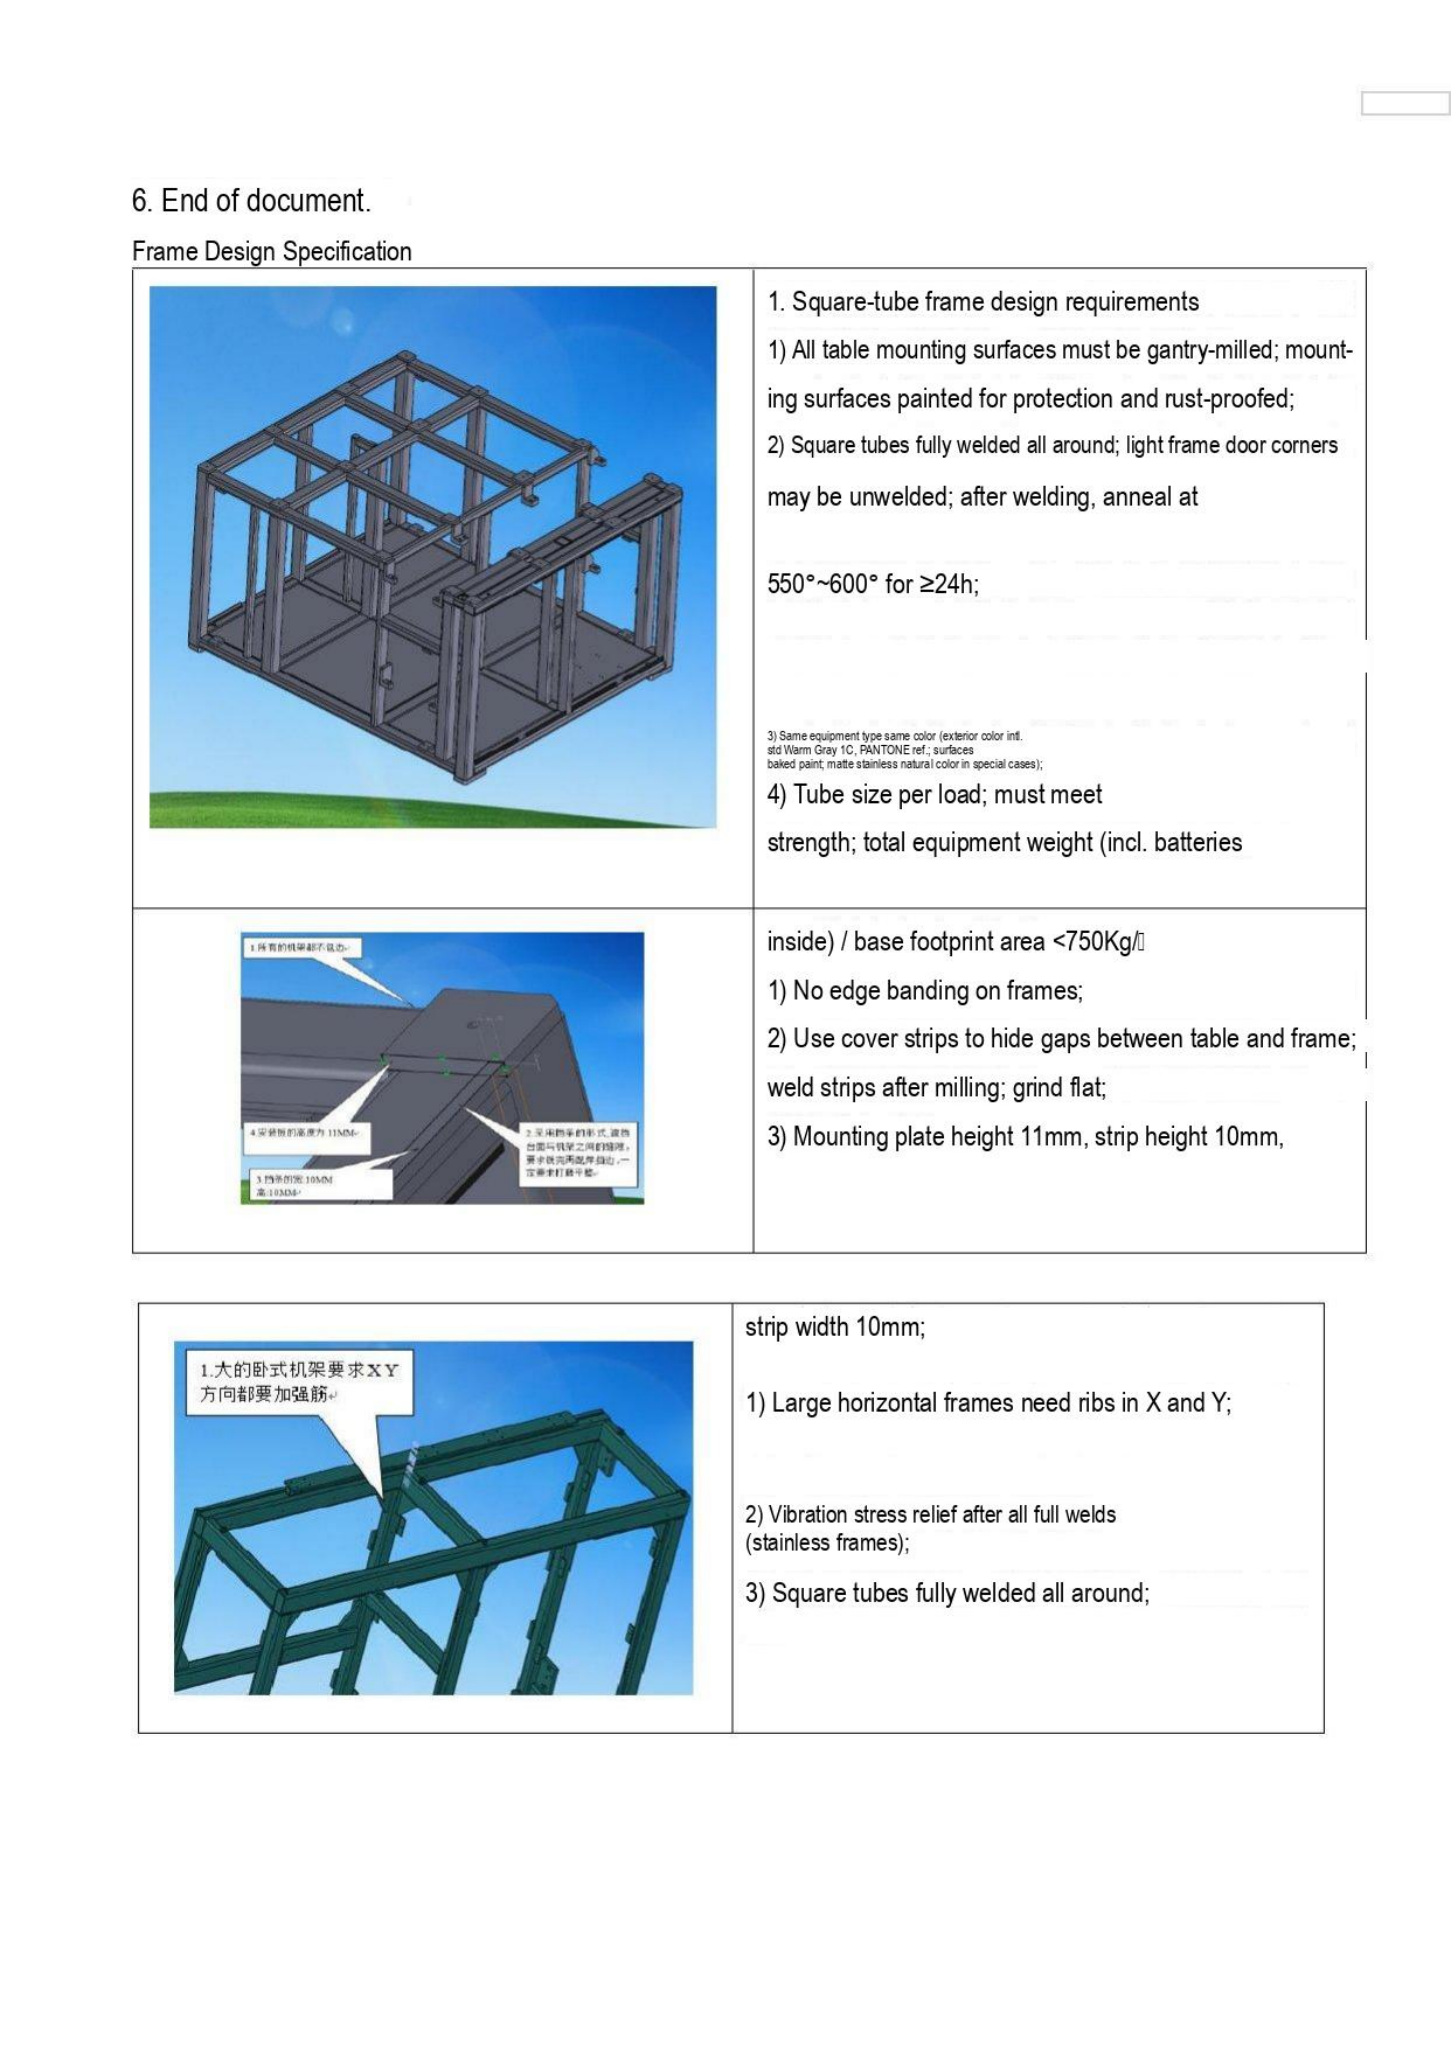6. End of document.

Frame Design Specification

| | |
|---|---|
| | 1. Square-tube frame design requirements<br>1) All table mounting surfaces must be gantry-milled; mounting surfaces painted for protection and rust-proofed;<br>2) Square tubes fully welded all around; light frame door corners may be unwelded; after welding, anneal at 550°~600° for ≥24h;<br>3) Same equipment type same color (exterior color inf. std Warm Gray 1C, PANTONE ref.; surfaces baked paint; matte stainless natural color in special cases);<br>4) Tube size per load; must meet strength; total equipment weight (incl. batteries |
| 1.所有的机架都不包边<br>4.安装板的高度为11MM<br>3.挡条的宽10MM 高10MM<br>2.采用挡条的形式,遮挡台面与机架之间的缝隙,要求铣完再焊挡条,一定要求打磨平整 | inside) / base footprint area <750Kg/<br>1) No edge banding on frames;<br>2) Use cover strips to hide gaps between table and frame; weld strips after milling; grind flat;<br>3) Mounting plate height 11mm, strip height 10mm, |

| | |
|---|---|
| 1.大的卧式机架要求XY方向都要加强筋 | strip width 10mm;<br>1) Large horizontal frames need ribs in X and Y;<br>2) Vibration stress relief after all full welds (stainless frames);<br>3) Square tubes fully welded all around; |
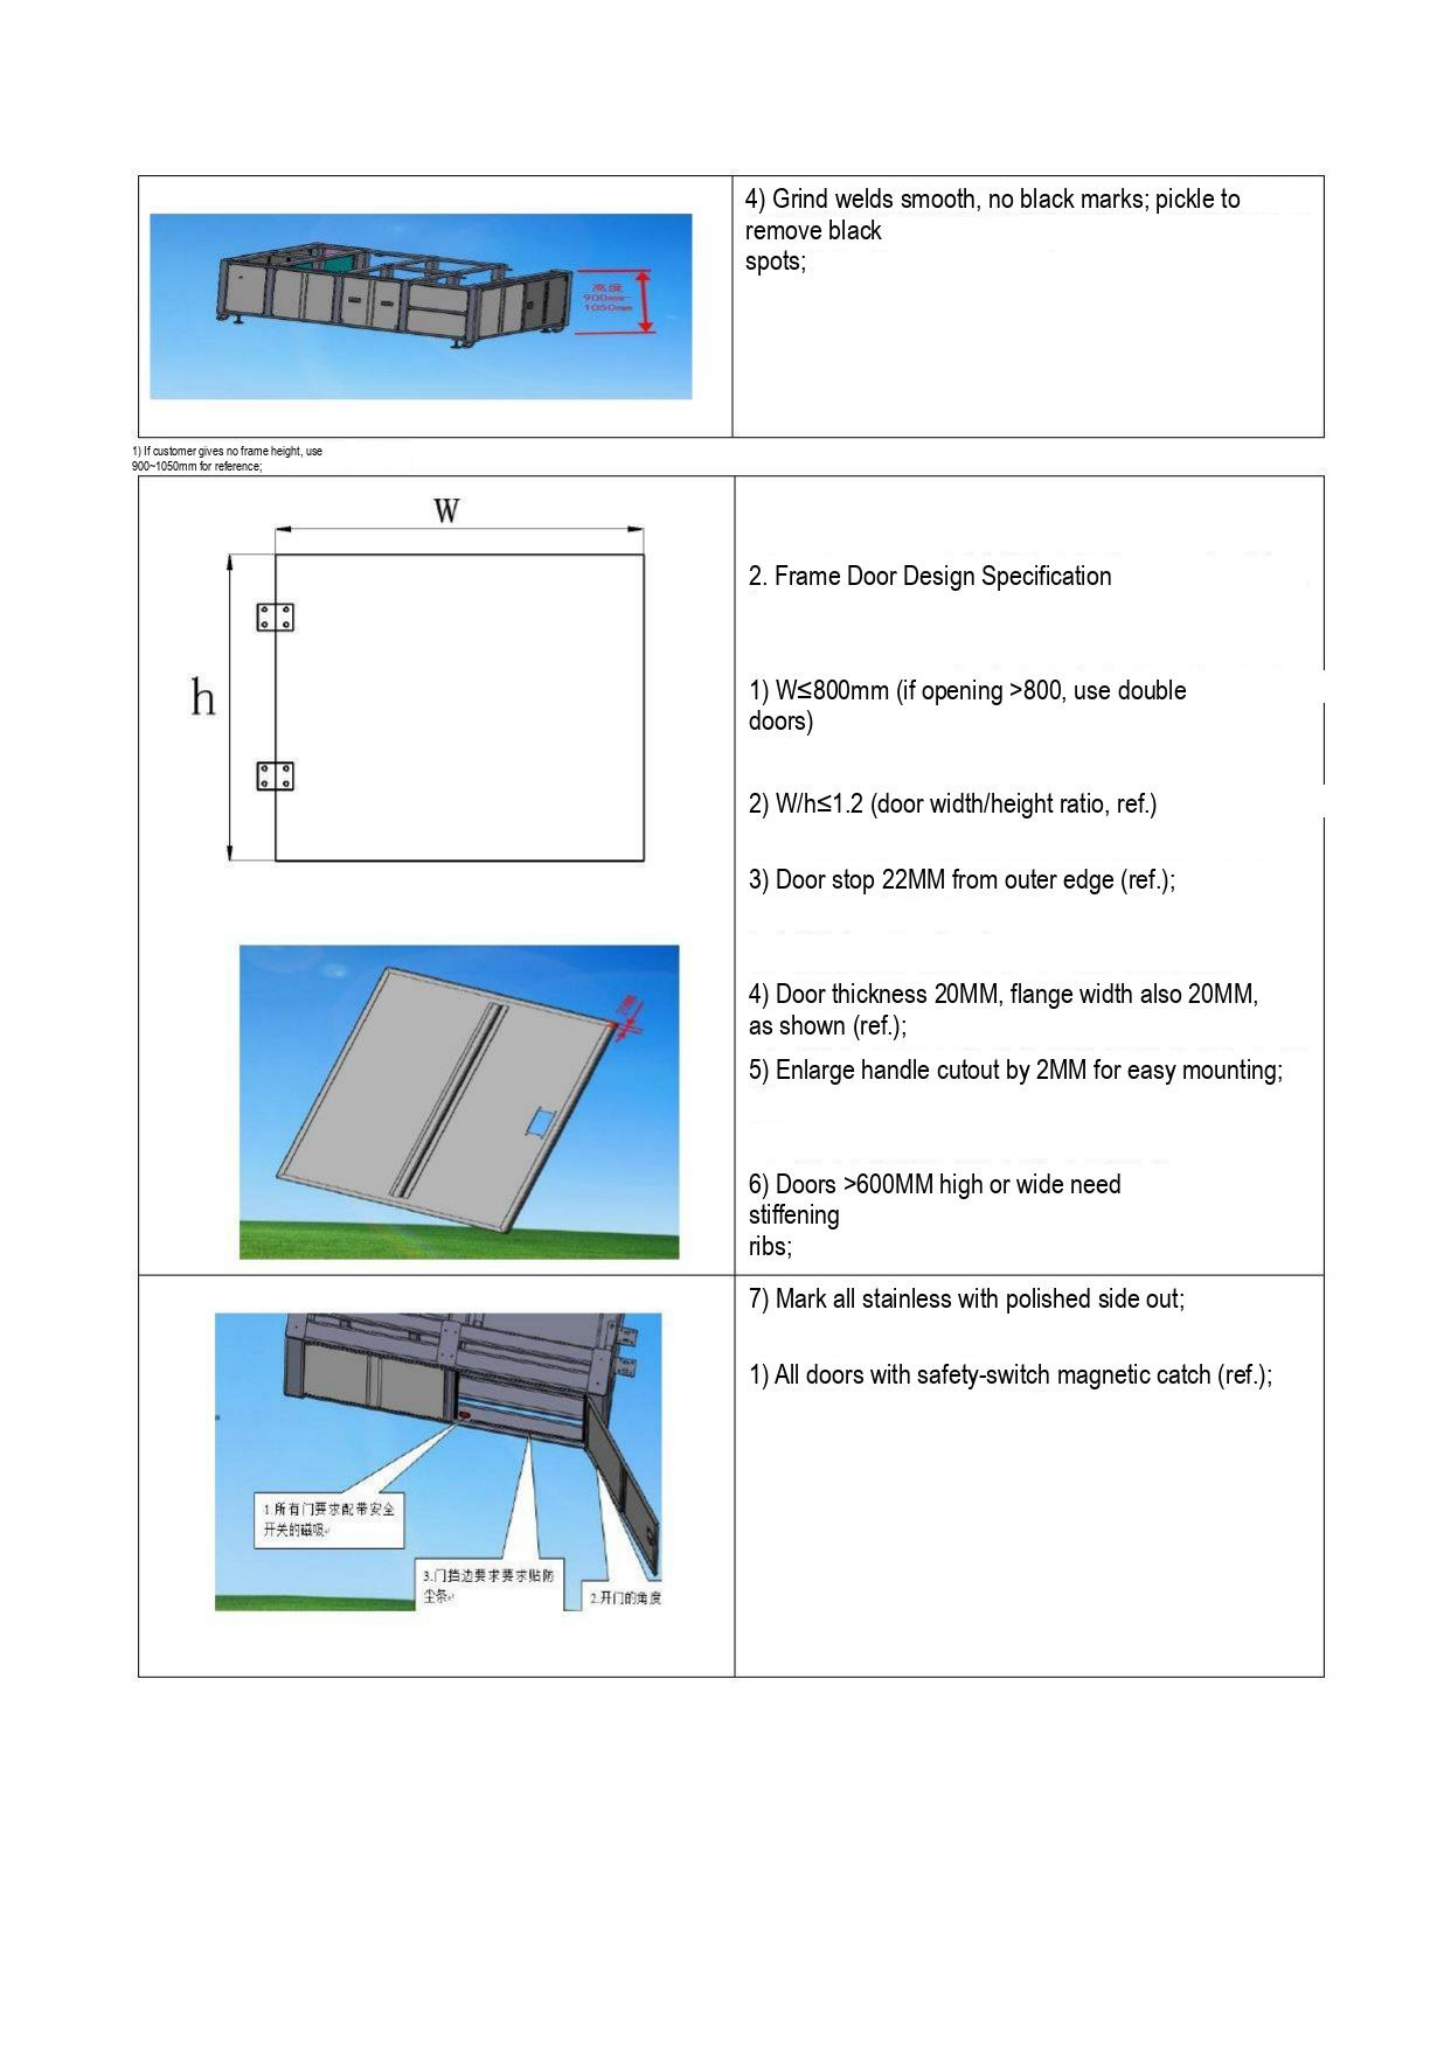| | |
|---|---|
| 高度 900mm~ 1050mm | 4) Grind welds smooth, no black marks; pickle to remove black spots; |

1) If customer gives no frame height, use 900~1050mm for reference;

| | |
|---|---|
| W<br>h | 2. Frame Door Design Specification<br><br>1) W≤800mm (if opening >800, use double doors)<br><br>2) W/h≤1.2 (door width/height ratio, ref.)<br><br>3) Door stop 22MM from outer edge (ref.);<br><br>4) Door thickness 20MM, flange width also 20MM, as shown (ref.);<br><br>5) Enlarge handle cutout by 2MM for easy mounting;<br><br>6) Doors >600MM high or wide need stiffening ribs; |
| 1.所有门要求配带安全开关的磁吸<br>3.门挡边要求要求贴防尘条<br>2.开门的角度 | 7) Mark all stainless with polished side out;<br><br>1) All doors with safety-switch magnetic catch (ref.); |
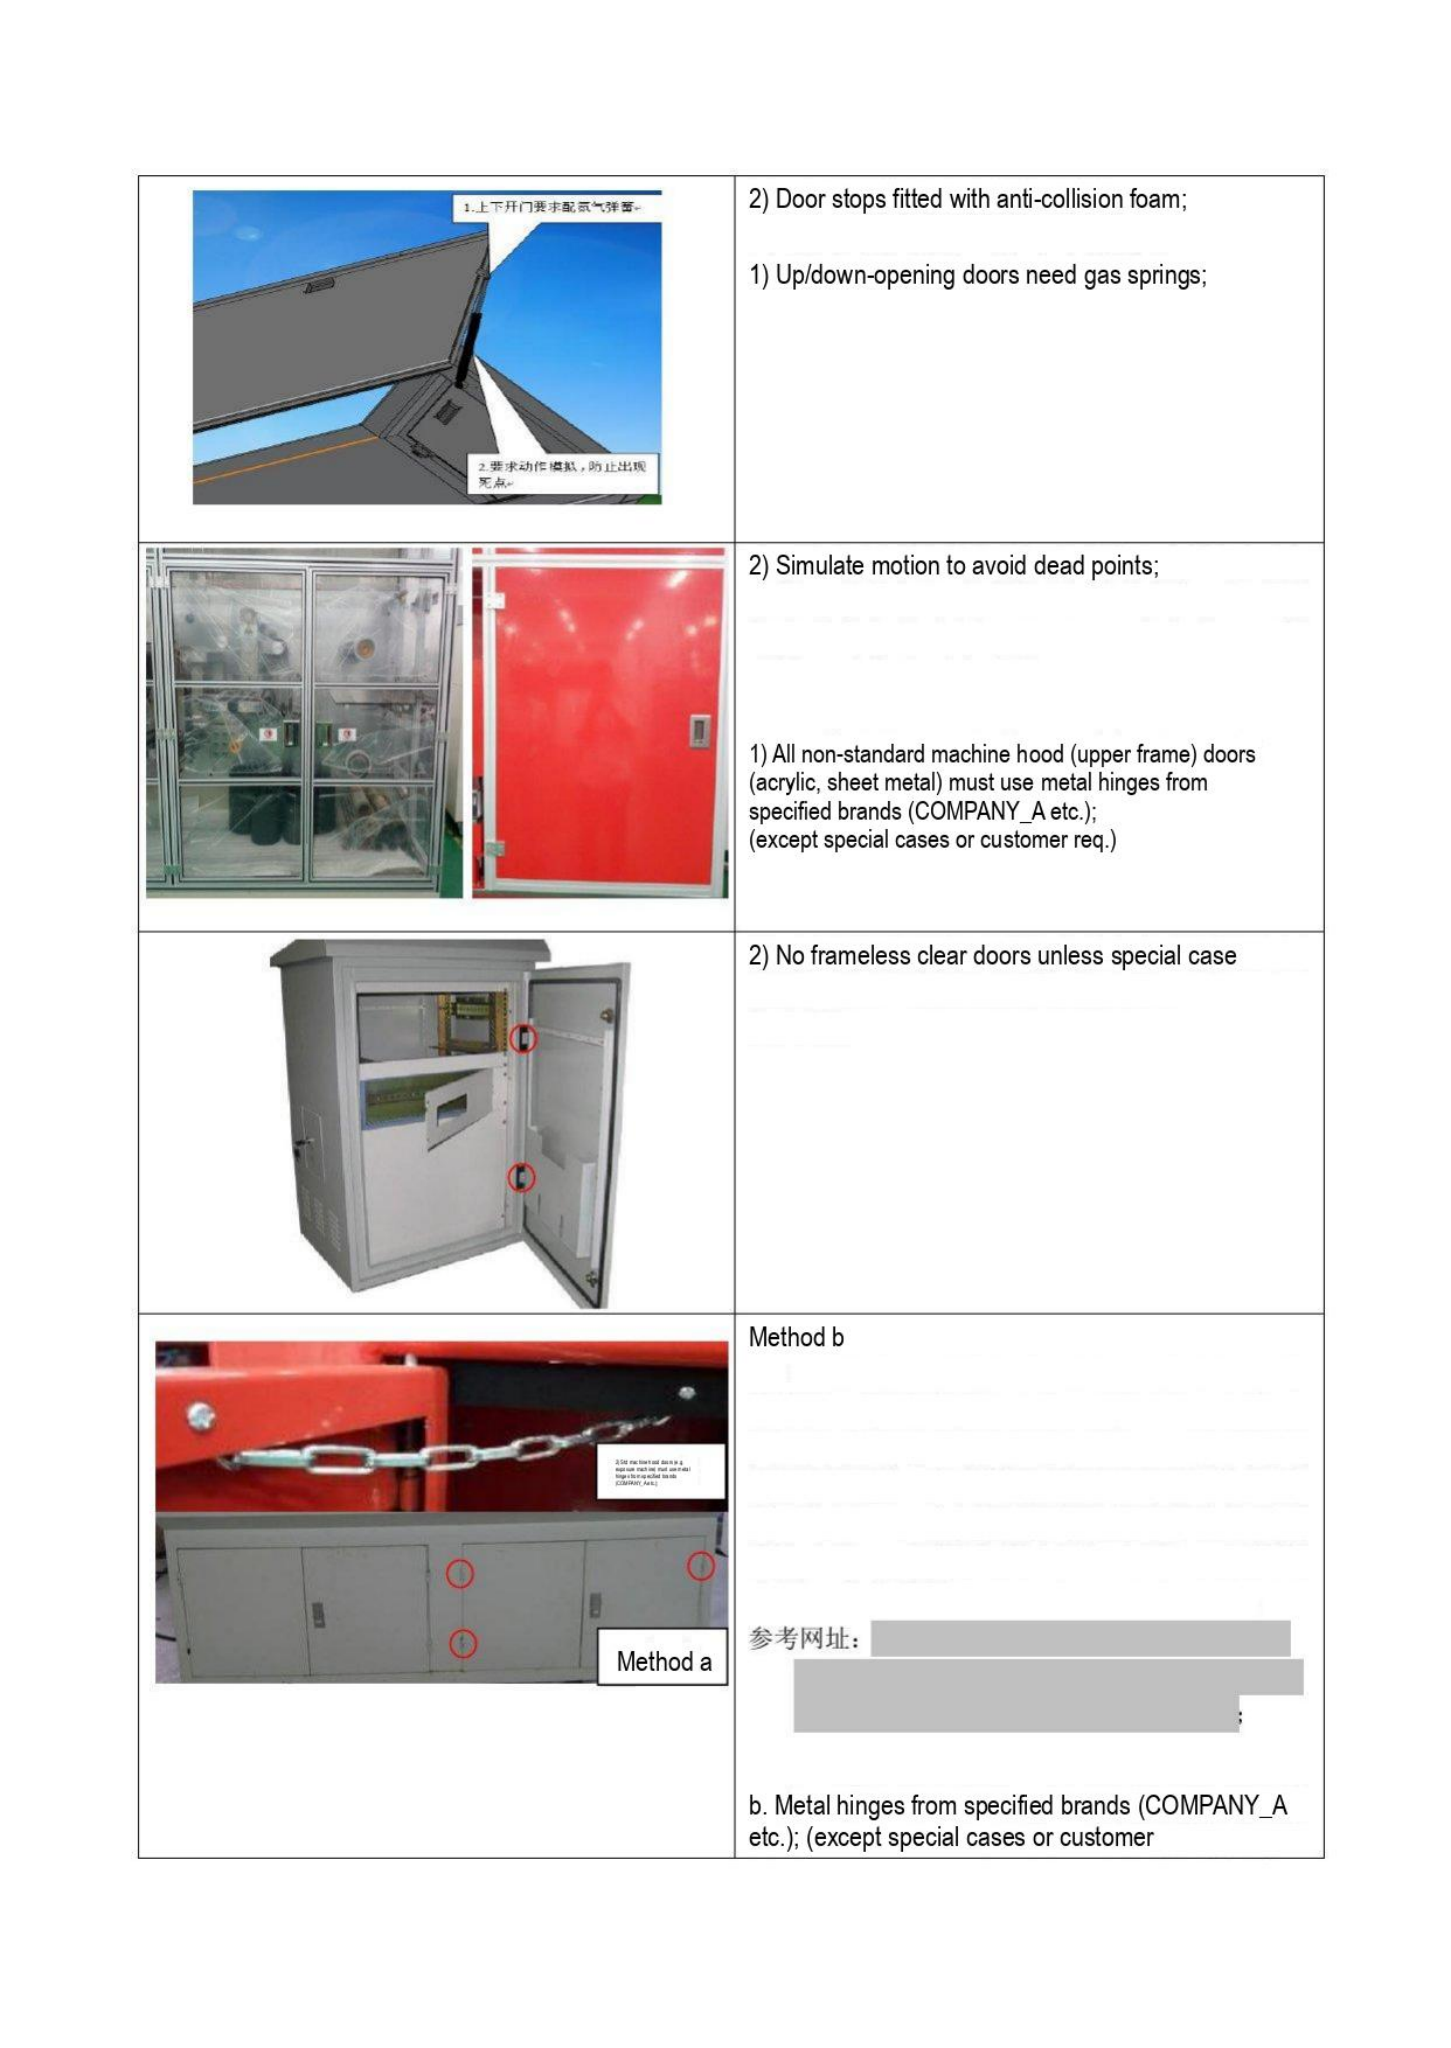| | |
|---|---|
| 1.上下开门要求配氮气弹簧<br>2.要求动作模拟，防止出现死点 | 2) Door stops fitted with anti-collision foam;<br><br>1) Up/down-opening doors need gas springs; |
| | 2) Simulate motion to avoid dead points;<br><br>1) All non-standard machine hood (upper frame) doors (acrylic, sheet metal) must use metal hinges from specified brands (COMPANY_A etc.);<br>(except special cases or customer req.) |
| | 2) No frameless clear doors unless special case |
| Method a | Method b<br><br>参考网址：<br><br>b. Metal hinges from specified brands (COMPANY_A etc.); (except special cases or customer |
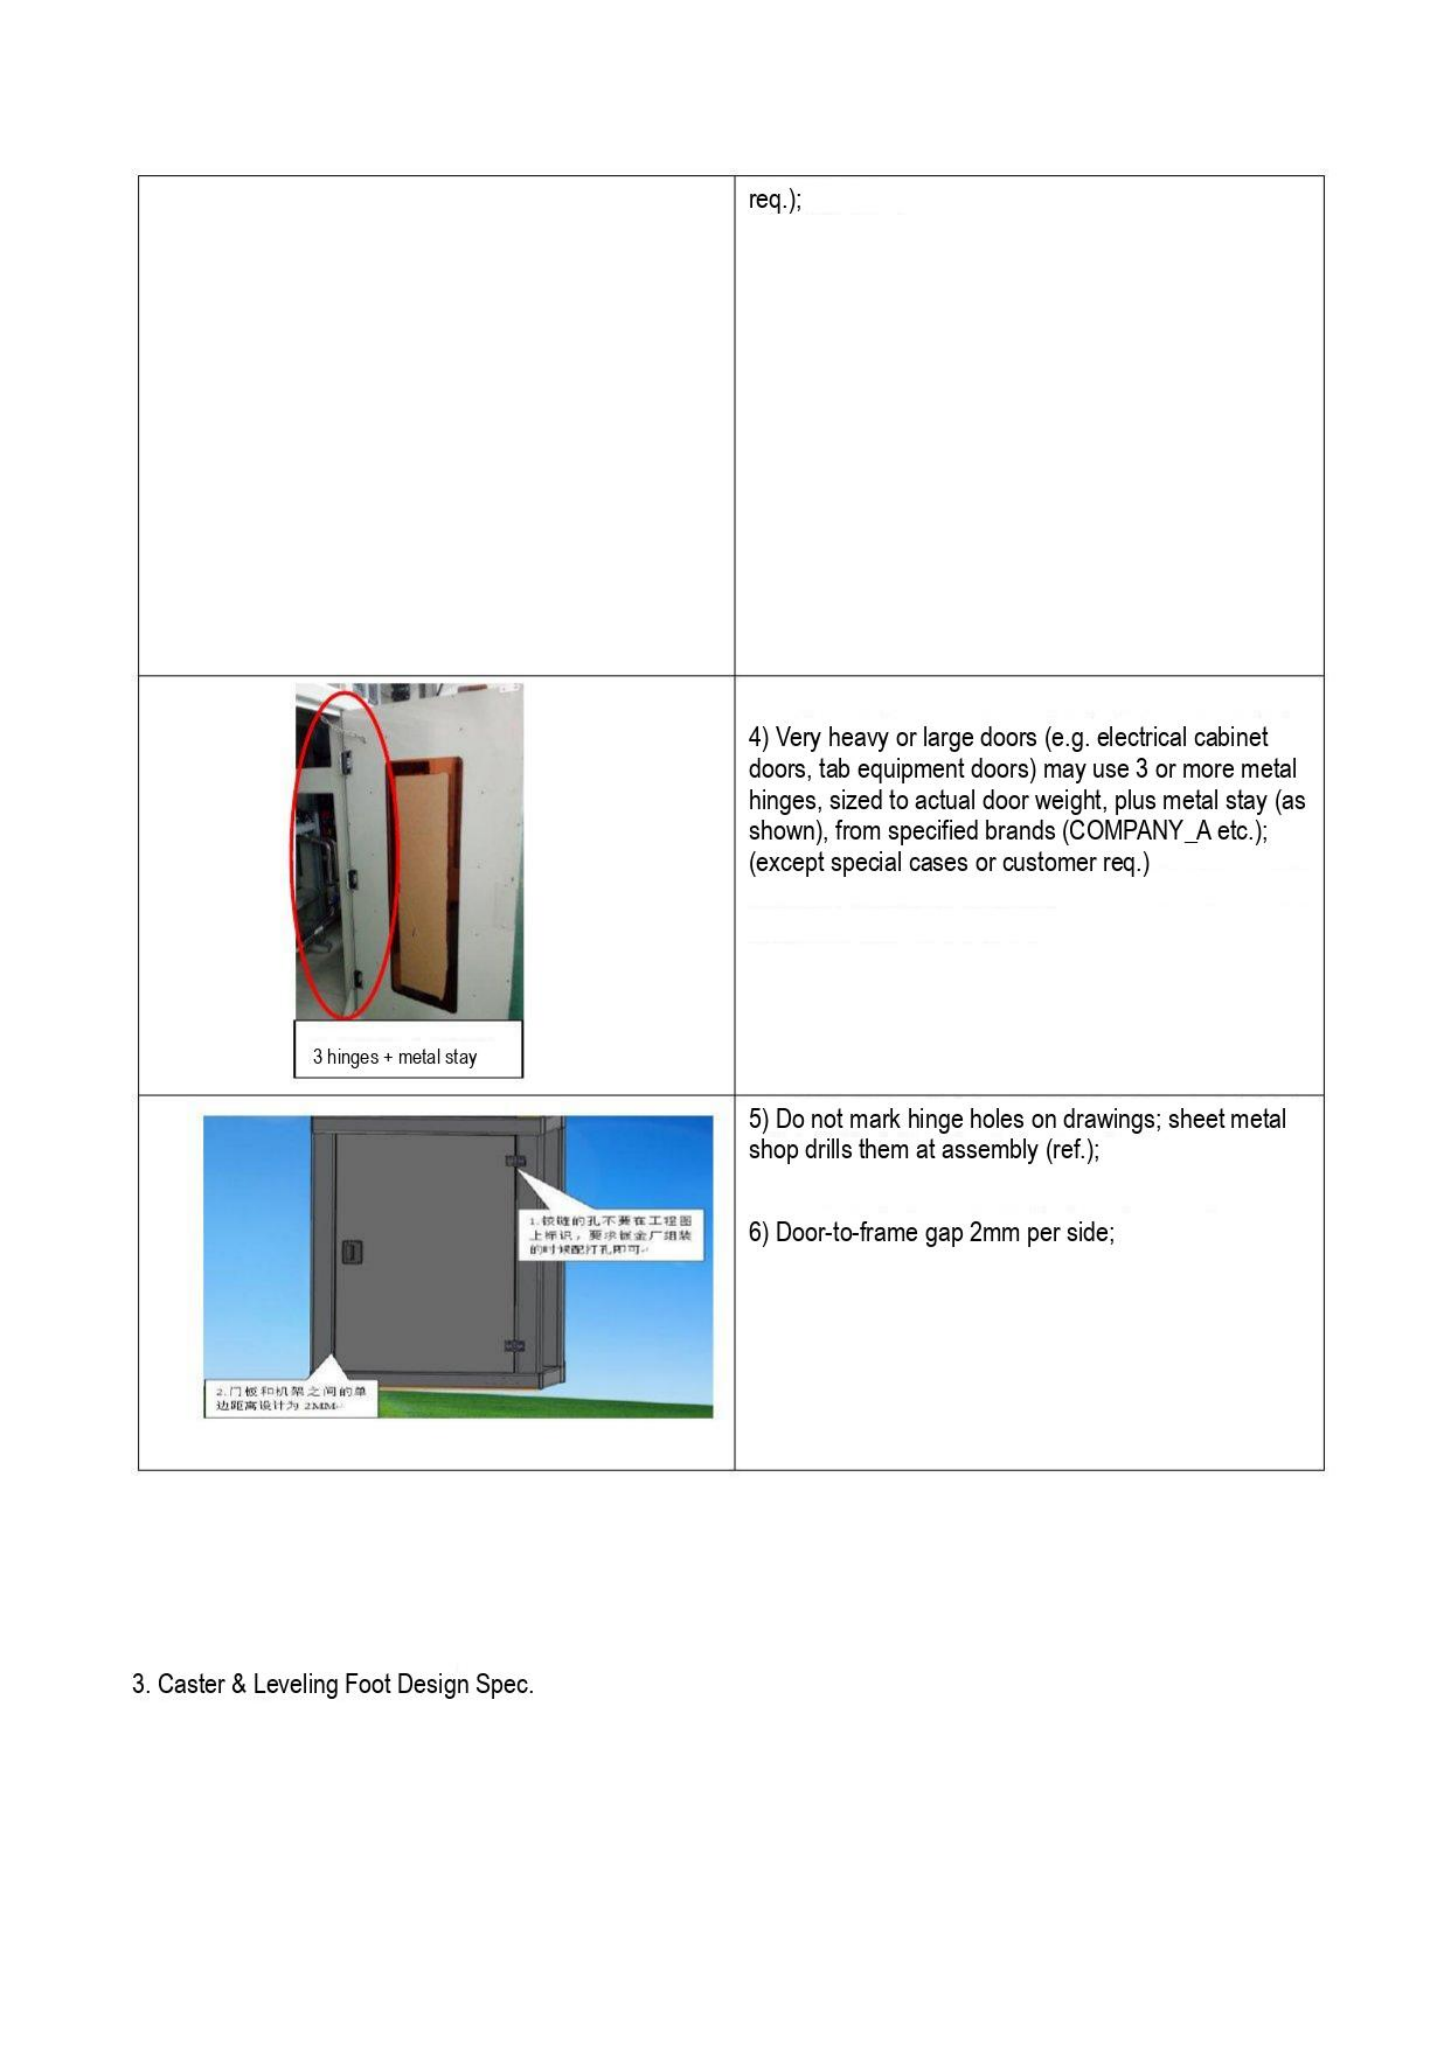| | |
|---|---|
| | req.); |
| 3 hinges + metal stay | 4) Very heavy or large doors (e.g. electrical cabinet doors, tab equipment doors) may use 3 or more metal hinges, sized to actual door weight, plus metal stay (as shown), from specified brands (COMPANY_A etc.); (except special cases or customer req.) |
| 1.铰链的孔不要在工程图上标识，要求钣金厂组装的时候配打孔即可<br>2.门板和机架之间的单边距离设计为2MM | 5) Do not mark hinge holes on drawings; sheet metal shop drills them at assembly (ref.);<br><br>6) Door-to-frame gap 2mm per side; |

3. Caster & Leveling Foot Design Spec.
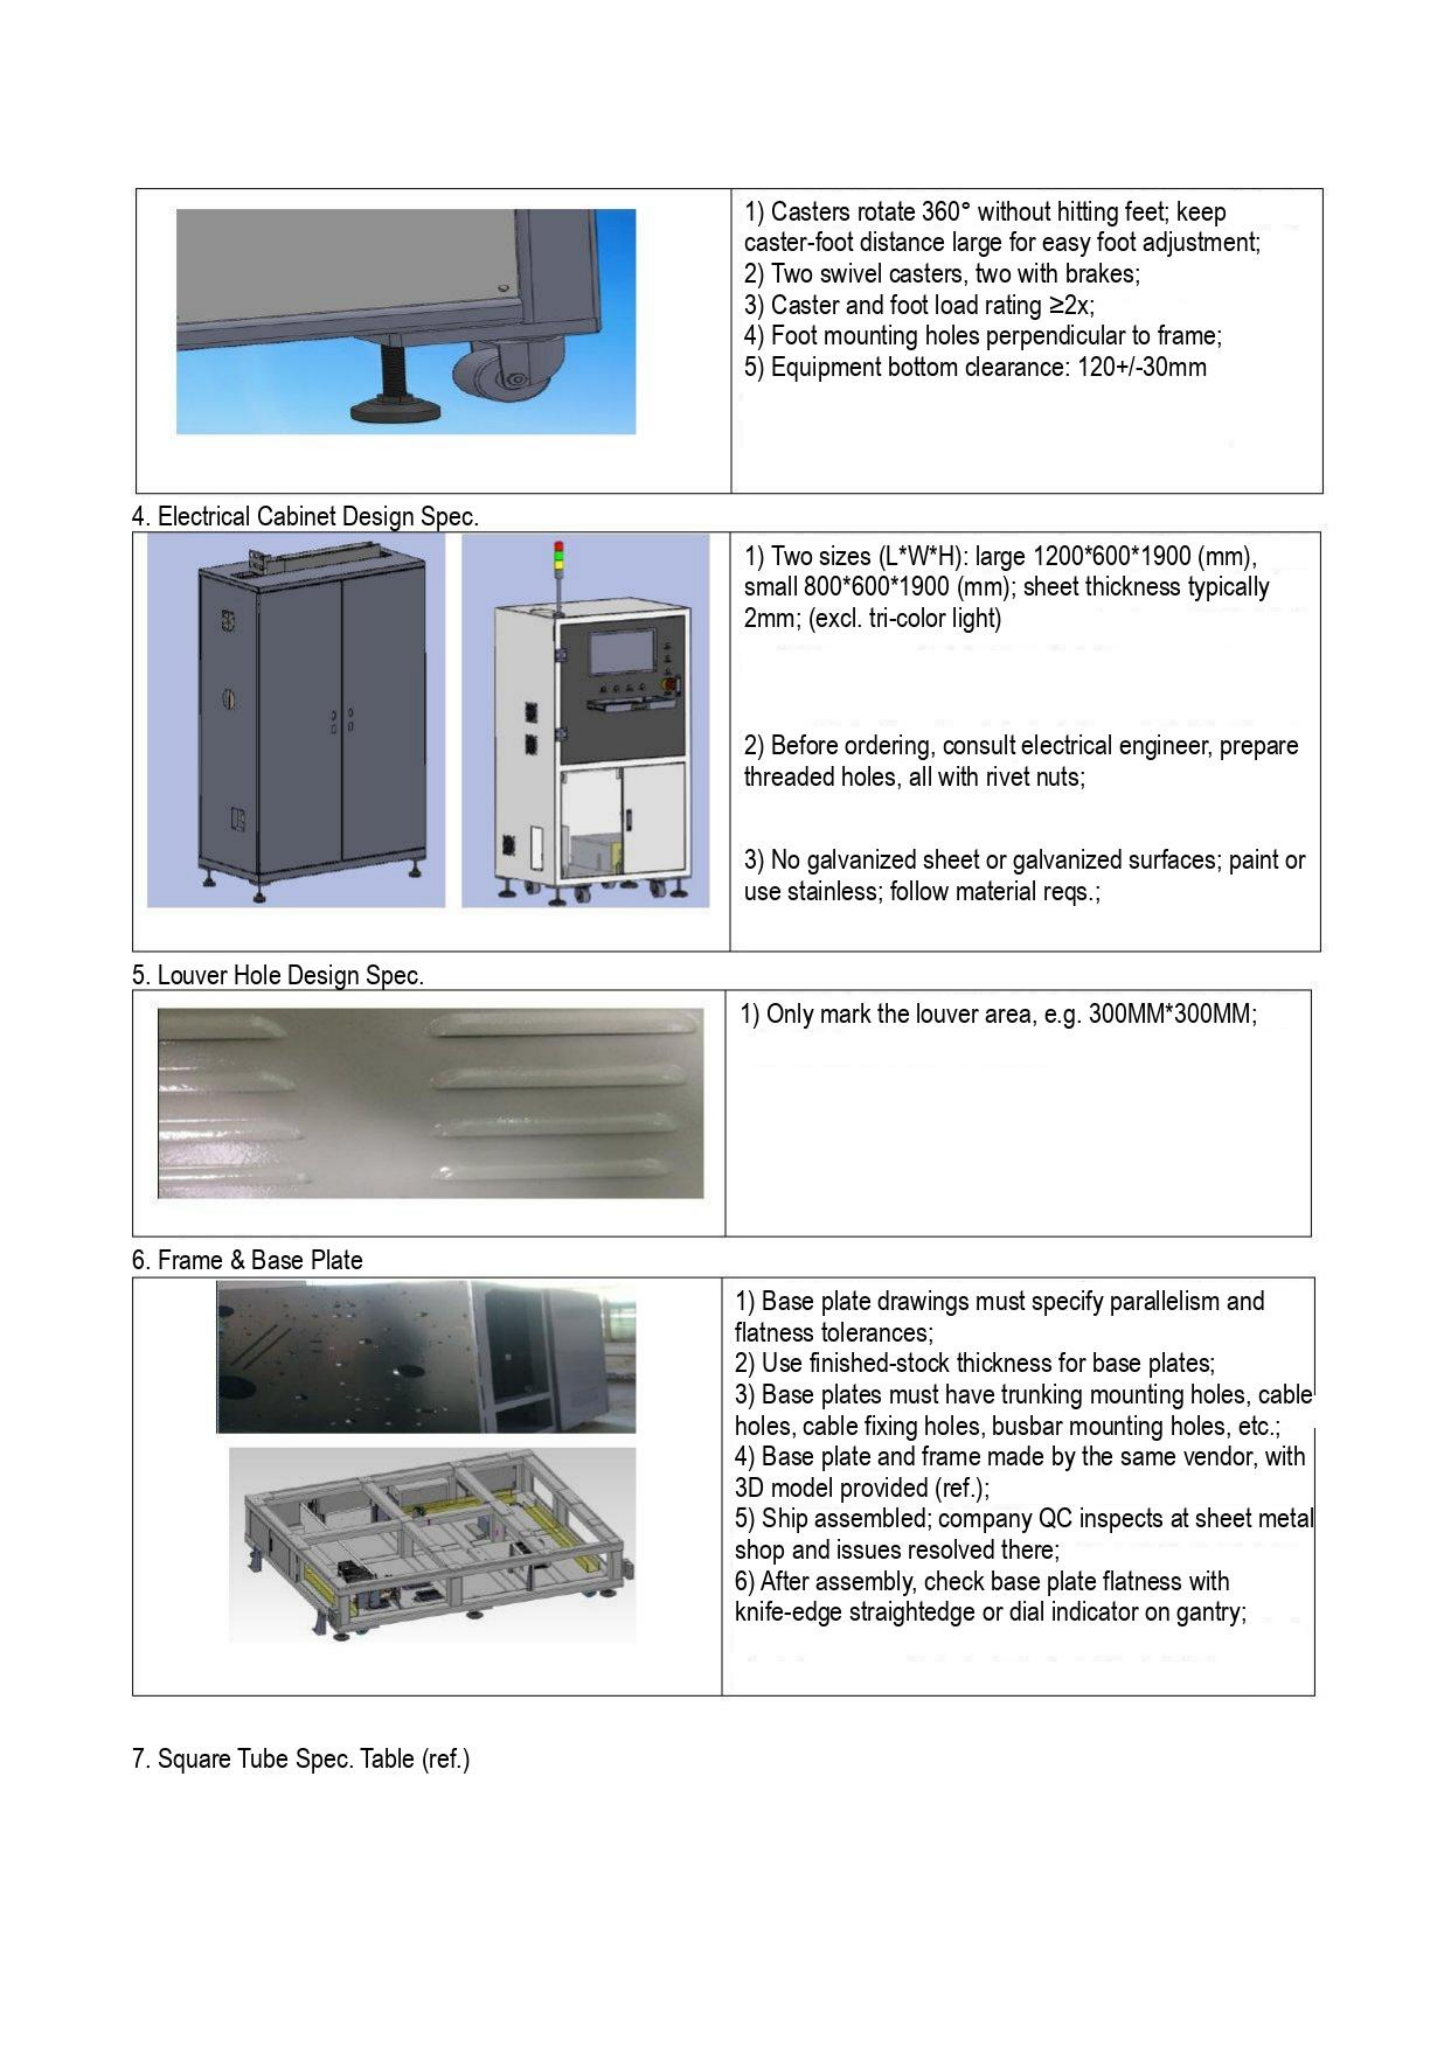| | |
|---|---|
| | 1) Casters rotate 360° without hitting feet; keep caster-foot distance large for easy foot adjustment;<br>2) Two swivel casters, two with brakes;<br>3) Caster and foot load rating ≥2x;<br>4) Foot mounting holes perpendicular to frame;<br>5) Equipment bottom clearance: 120+/-30mm |

4. Electrical Cabinet Design Spec.

| | |
|---|---|
| | 1) Two sizes (L\*W\*H): large 1200\*600\*1900 (mm), small 800\*600\*1900 (mm); sheet thickness typically 2mm; (excl. tri-color light)<br><br>2) Before ordering, consult electrical engineer, prepare threaded holes, all with rivet nuts;<br><br>3) No galvanized sheet or galvanized surfaces; paint or use stainless; follow material reqs.; |

5. Louver Hole Design Spec.

| | |
|---|---|
| | 1) Only mark the louver area, e.g. 300MM\*300MM; |

6. Frame & Base Plate

| | |
|---|---|
| | 1) Base plate drawings must specify parallelism and flatness tolerances;<br>2) Use finished-stock thickness for base plates;<br>3) Base plates must have trunking mounting holes, cable holes, cable fixing holes, busbar mounting holes, etc.;<br>4) Base plate and frame made by the same vendor, with 3D model provided (ref.);<br>5) Ship assembled; company QC inspects at sheet metal shop and issues resolved there;<br>6) After assembly, check base plate flatness with knife-edge straightedge or dial indicator on gantry; |

7. Square Tube Spec. Table (ref.)
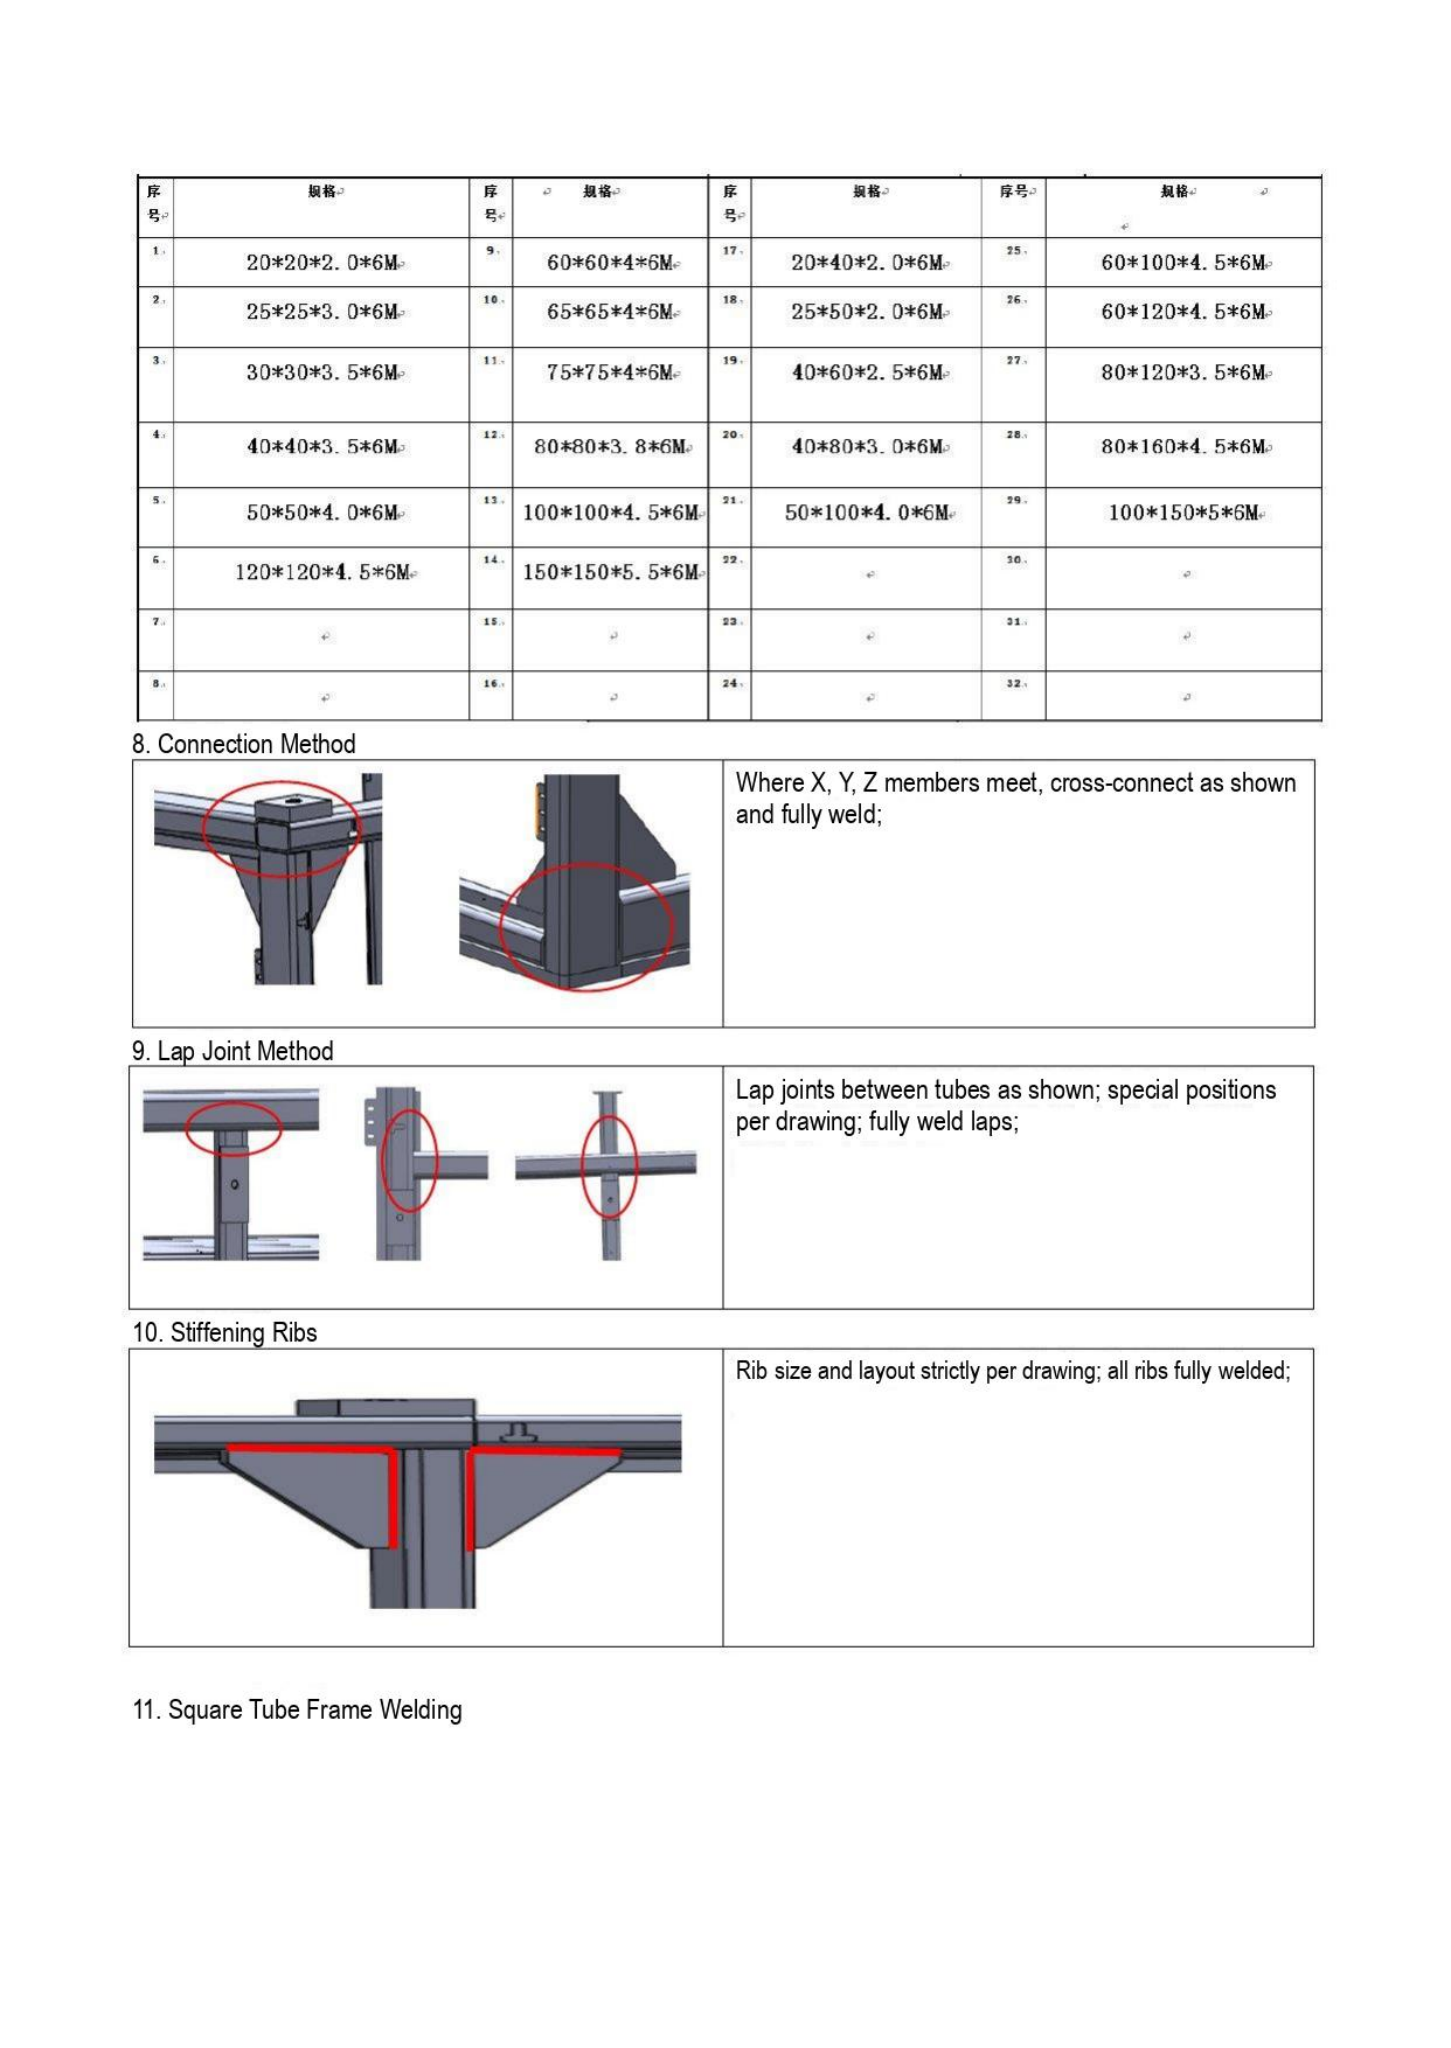| 序号 | 规格 | 序号 | 规格 | 序号 | 规格 | 序号 | 规格 |
|---|---|---|---|---|---|---|---|
| 1 | 20*20*2.0*6M | 9 | 60*60*4*6M | 17 | 20*40*2.0*6M | 25 | 60*100*4.5*6M |
| 2 | 25*25*3.0*6M | 10 | 65*65*4*6M | 18 | 25*50*2.0*6M | 26 | 60*120*4.5*6M |
| 3 | 30*30*3.5*6M | 11 | 75*75*4*6M | 19 | 40*60*2.5*6M | 27 | 80*120*3.5*6M |
| 4 | 40*40*3.5*6M | 12 | 80*80*3.8*6M | 20 | 40*80*3.0*6M | 28 | 80*160*4.5*6M |
| 5 | 50*50*4.0*6M | 13 | 100*100*4.5*6M | 21 | 50*100*4.0*6M | 29 | 100*150*5*6M |
| 6 | 120*120*4.5*6M | 14 | 150*150*5.5*6M | 22 | | 30 | |
| 7 | | 15 | | 23 | | 31 | |
| 8 | | 16 | | 24 | | 32 | |

8. Connection Method

| | |
|---|---|
| | Where X, Y, Z members meet, cross-connect as shown and fully weld; |

9. Lap Joint Method

| | |
|---|---|
| | Lap joints between tubes as shown; special positions per drawing; fully weld laps; |

10. Stiffening Ribs

| | |
|---|---|
| | Rib size and layout strictly per drawing; all ribs fully welded; |

11. Square Tube Frame Welding
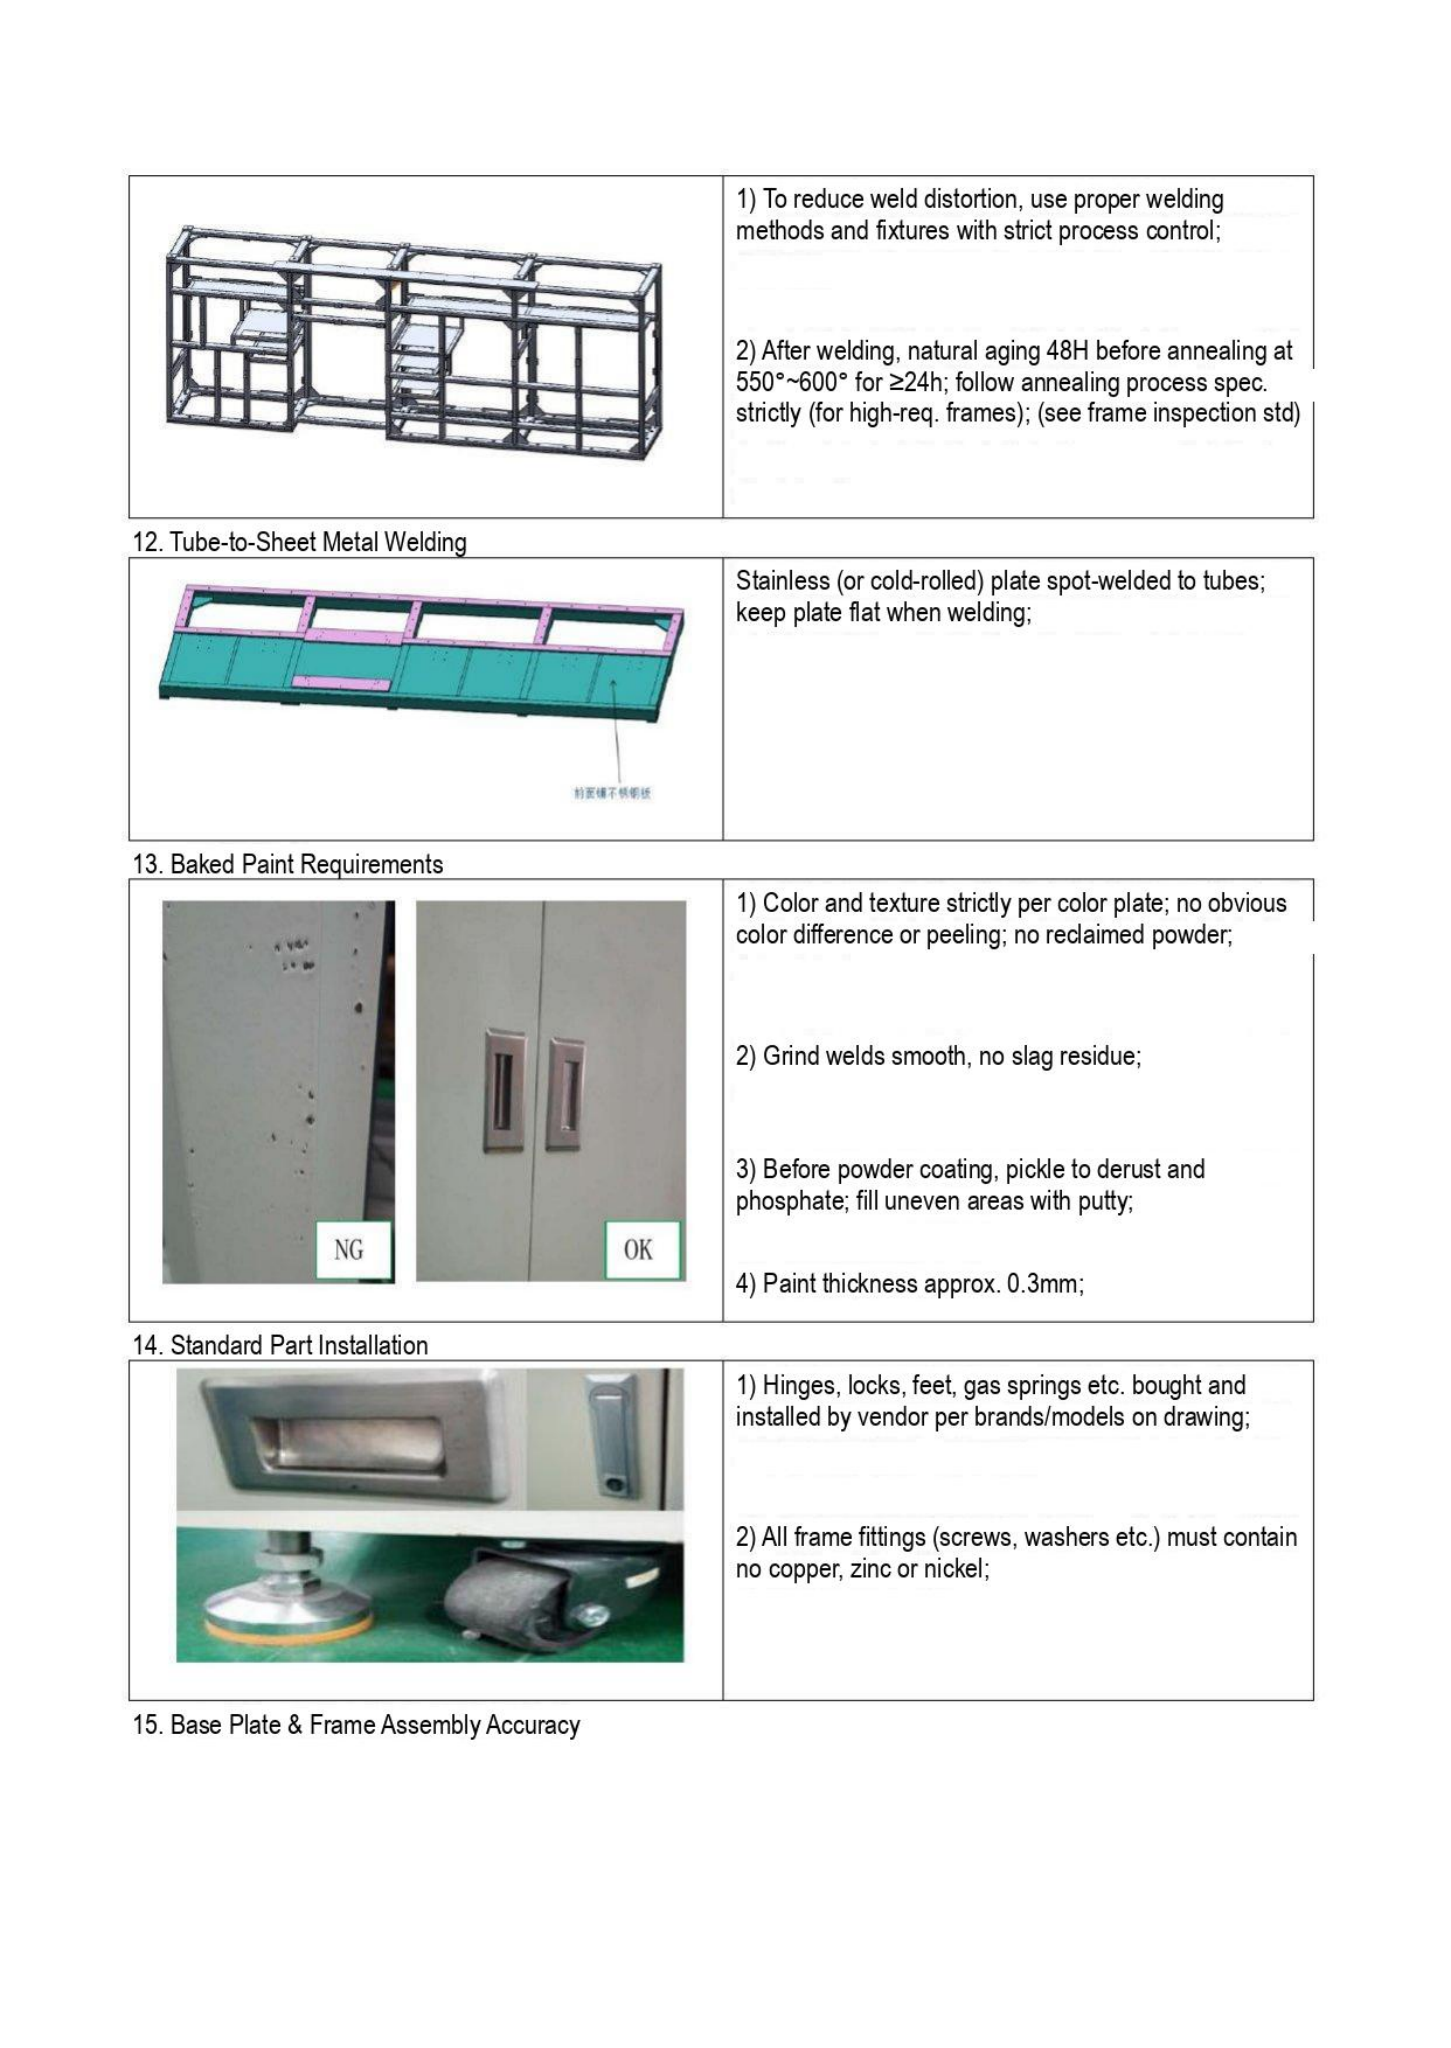| | |
|---|---|
| | 1) To reduce weld distortion, use proper welding methods and fixtures with strict process control;<br><br>2) After welding, natural aging 48H before annealing at 550°~600° for ≥24h; follow annealing process spec. strictly (for high-req. frames); (see frame inspection std) |

12. Tube-to-Sheet Metal Welding

| | |
|---|---|
| | Stainless (or cold-rolled) plate spot-welded to tubes; keep plate flat when welding; |

13. Baked Paint Requirements

| | |
|---|---|
| NG OK | 1) Color and texture strictly per color plate; no obvious color difference or peeling; no reclaimed powder;<br><br>2) Grind welds smooth, no slag residue;<br><br>3) Before powder coating, pickle to derust and phosphate; fill uneven areas with putty;<br><br>4) Paint thickness approx. 0.3mm; |

14. Standard Part Installation

| | |
|---|---|
| | 1) Hinges, locks, feet, gas springs etc. bought and installed by vendor per brands/models on drawing;<br><br>2) All frame fittings (screws, washers etc.) must contain no copper, zinc or nickel; |

15. Base Plate & Frame Assembly Accuracy